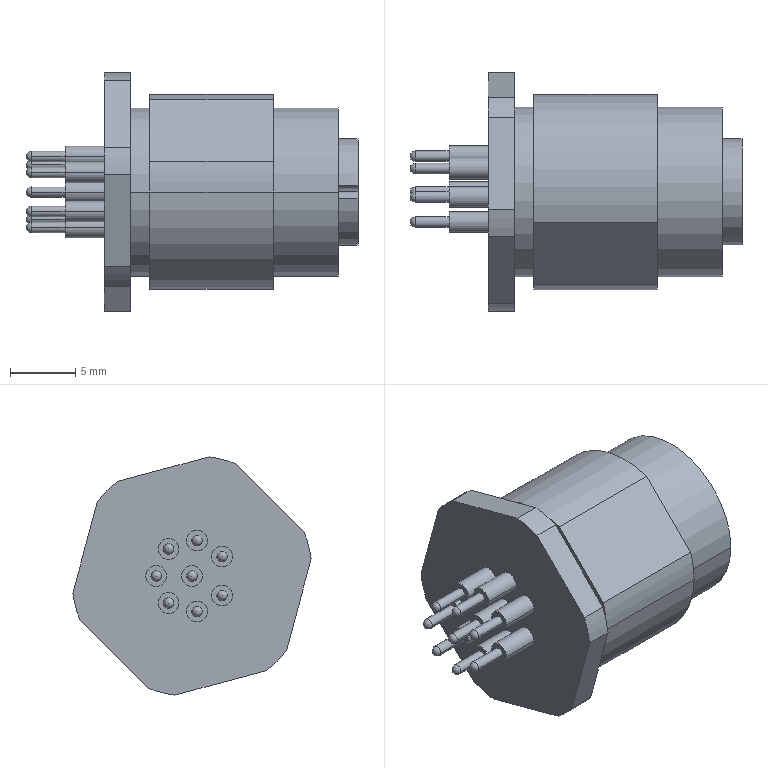Part | NX | features BREP 1 | 1 solid | 107 faces | box 25.5 x 18.309 x 18.309 mm | volume 2671 mm3 | cylinder 66 | plane 33 | sphere 8 | commonest cylinder face diameters 0.7 x16 0.8 x16 1.6 x16 18.5 x6 13 x4 15 x3